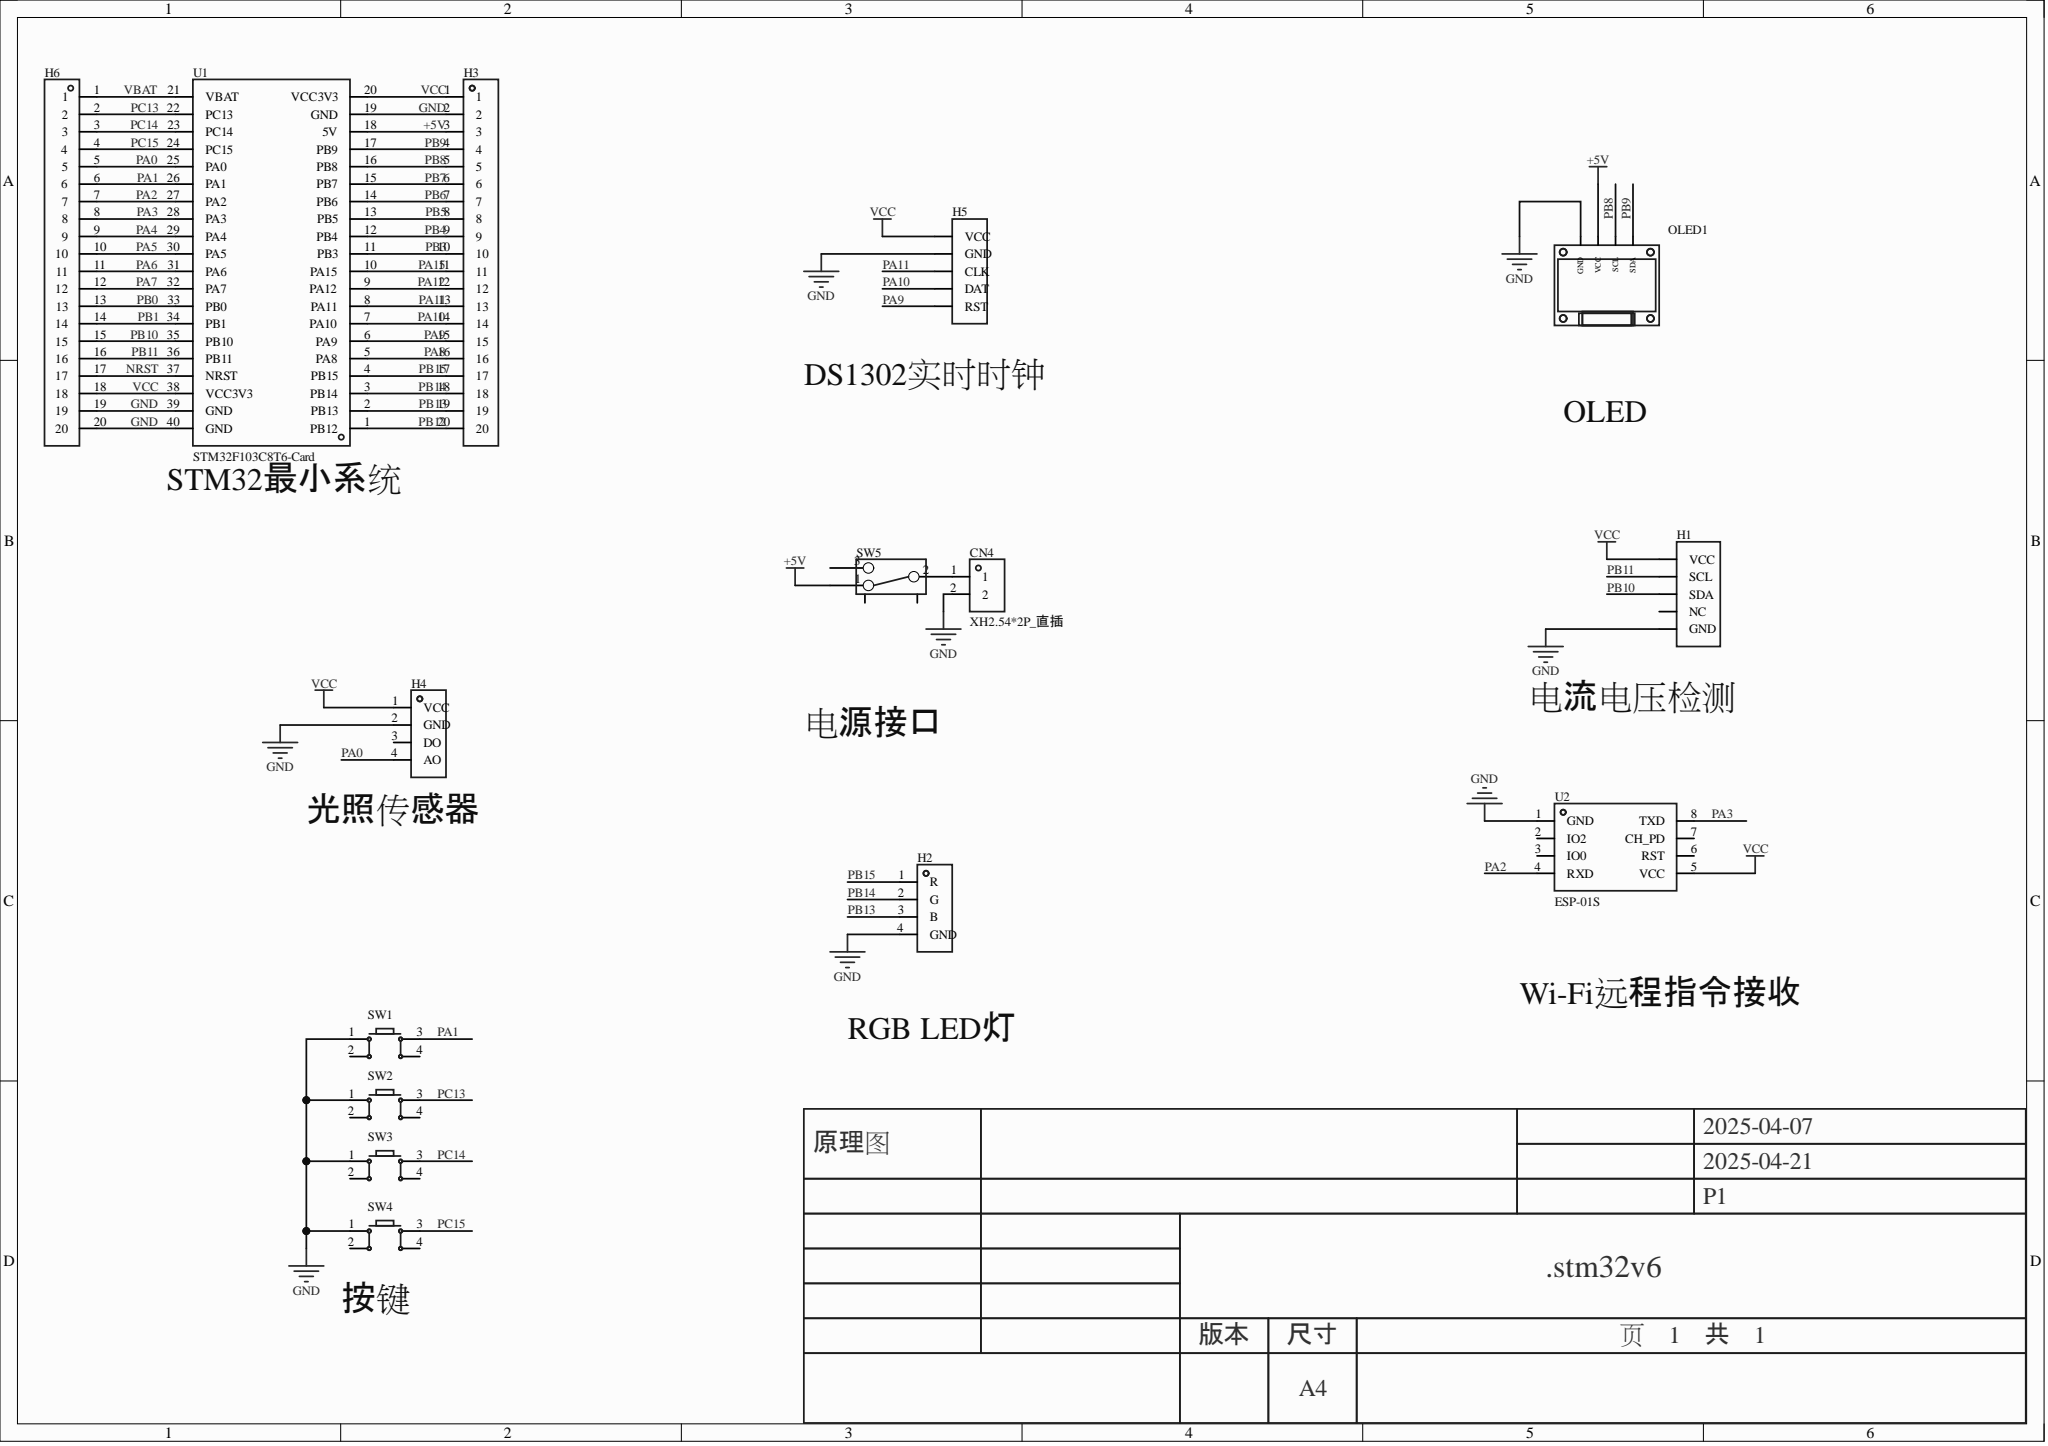Circuit board | Altium Designer | 15 parts | 38 nets
Bill of materials:
Comment,Description,Designator,Footprint,LibRef,Quantity
"XH2.54*2P_直插","","CN4","CONN-TH_2P-P2.50-XH2.54-2P","XH2.54*2P_直插","1"
"","","H1, H5","HDR-TH_5P-P2.54-V-F","HDR-F_2.54_1x5P","2"
"","","H2, H4","HDR-TH_4P-P2.54-V-F","HDR-F_2.54_1x4P","2"
"","间距:2.54mm;总PIN位数:20;排数:1;插针结构:-;行距:-;安装类型:直插;圆针/方针:-;额定电流:-;额定电压:-;配合针长度:-;塑高:-;触头材质:黄铜;触头镀层:-;颜色:黑色;","H3, H6","HDR-TH_20P-P2.54-V-M-1","HDR-M_2.54_1x20P","2"
"","","OLED1","0.96OLED_4P","0.96OLED模块_4P","1"
"","","SW1, SW2, SW3, SW4","SW-TH_4P-L6.0-W6.0-P4.50-LS6.5","Key_TH_6x6x6","4"
"","","SW5","拨动开关","拨动开关_正","1"
"STM32F103C8T6-Card","","U1","CONN-TH_L53.3-W22.9_STM32F103C8T6-CARD","STM32F103C8T6-Card","1"
"ESP-01S","","U2","WIFIM-TH_ESP-01S","ESP-01S_C111009","1"
Netlist (Protel format):
[
CN4
CONN-TH_2P-P2.50-XH2.54-2P
XH2.54*2P_直插



]
[
H1
HDR-TH_5P-P2.54-V-F




]
[
H2
HDR-TH_4P-P2.54-V-F




]
[
H3
HDR-TH_20P-P2.54-V-M-1




]
[
H4
HDR-TH_4P-P2.54-V-F




]
[
H5
HDR-TH_5P-P2.54-V-F




]
[
H6
HDR-TH_20P-P2.54-V-M-1




]
[
OLED1
0.96OLED_4P




]
[
SW1
SW-TH_4P-L6.0-W6.0-P4.50-LS6.5




]
[
SW2
SW-TH_4P-L6.0-W6.0-P4.50-LS6.5




]
[
SW3
SW-TH_4P-L6.0-W6.0-P4.50-LS6.5




]
[
SW4
SW-TH_4P-L6.0-W6.0-P4.50-LS6.5




]
[
SW5
拨动开关




]
[
U1
CONN-TH_L53.3-W22.9_STM32F103C8T6-CARD
STM32F103C8T6-Card



]
[
U2
WIFIM-TH_ESP-01S
ESP-01S



]
(
VCC
H1-1
H3-1
H4-1
H5-1
H6-18
U1-20
U1-38
U2-5
)
(
VBAT
H6-1
U1-21
)
(
PC15
H6-4
SW4-3
U1-24
)
(
PC14
H6-3
SW3-3
U1-23
)
(
PC13
H6-2
SW2-3
U1-22
)
(
PB15
H2-1
H3-17
U1-4
)
(
PB14
H2-2
H3-18
U1-3
)
(
PB13
H2-3
H3-19
U1-2
)
(
PB12
H3-20
U1-1
)
(
PB11
H1-2
H6-16
U1-36
)
(
PB10
H1-3
H6-15
U1-35
)
(
PB9
H3-4
OLED1-4
U1-17
)
(
PB8
H3-5
OLED1-3
U1-16
)
(
PB7
H3-6
U1-15
)
(
PB6
H3-7
U1-14
)
(
PB5
H3-8
U1-13
)
(
PB4
H3-9
U1-12
)
(
PB3
H3-10
U1-11
)
(
PB1
H6-14
U1-34
)
(
PB0
H6-13
U1-33
)
(
PA15
H3-11
U1-10
)
(
PA12
H3-12
U1-9
)
(
PA11
H3-13
H5-3
U1-8
)
(
PA10
H3-14
H5-4
U1-7
)
(
PA9
H3-15
H5-5
U1-6
)
(
PA8
H3-16
U1-5
)
(
PA7
H6-12
U1-32
)
(
PA6
H6-11
U1-31
)
(
PA5
H6-10
U1-30
)
(
PA4
H6-9
U1-29
)
(
PA3
H6-8
U1-28
U2-8
)
(
PA2
H6-7
U1-27
U2-4
)
(
PA1
H6-6
SW1-3
U1-26
)
(
PA0
H4-4
H6-5
U1-25
)
(
NRST
H6-17
U1-37
)
(
NetCN4_1
CN4-1
SW5-2
)
(
GND
CN4-2
H1-5
H2-4
H3-2
H4-2
H5-2
H6-19
H6-20
OLED1-1
SW1-1
SW2-1
SW3-1
SW4-1
U1-19
U1-39
U1-40
U2-1
)
(
+5V
H3-3
OLED1-2
SW5-1
U1-18
)